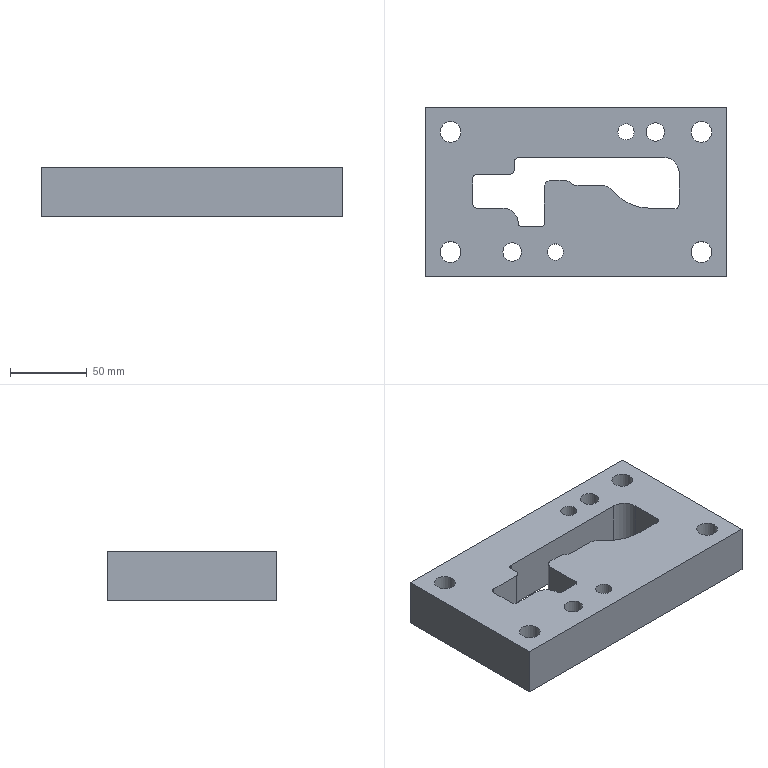Part | STEP file | lll_id226_x_t | 1 solid | 49 faces | box 195 x 110 x 32 mm | volume 531719 mm3 | cylinder 27 | plane 22 | commonest cylinder face diameters 6 x6 13.509 x4 20.008 x4 4 x2 8 x2 10.505 x2
STEP:
#1=CARTESIAN_POINT('',(1138.753,9.,60.5));
#2=VERTEX_POINT('',#1);
#3=CARTESIAN_POINT('',(1133.5,9.,60.5));
#4=DIRECTION('',(0.,0.,1.));
#5=DIRECTION('',(1.,0.,0.));
#6=AXIS2_PLACEMENT_3D('',#3,#4,#5);
#7=CIRCLE('',#6,5.253);
#8=EDGE_CURVE('',#2,#2,#7,.T.);
#9=ORIENTED_EDGE('',*,*,#8,.T.);
#10=EDGE_LOOP('',(#9));
#11=FACE_BOUND('',#10,.T.);
#12=CARTESIAN_POINT('',(1065.5,-69.,60.5));
#13=VERTEX_POINT('',#12);
#14=CARTESIAN_POINT('',(1059.5,-69.,60.5));
#15=DIRECTION('',(0.,0.,-1.));
#16=DIRECTION('',(1.,0.,0.));
#17=AXIS2_PLACEMENT_3D('',#14,#15,#16);
#18=CIRCLE('',#17,6.);
#19=EDGE_CURVE('',#13,#13,#18,.T.);
#20=ORIENTED_EDGE('',*,*,#19,.F.);
#21=EDGE_LOOP('',(#20));
#22=FACE_BOUND('',#21,.T.);
#23=CARTESIAN_POINT('',(1158.5,9.,60.5));
#24=VERTEX_POINT('',#23);
#25=CARTESIAN_POINT('',(1152.5,9.,60.5));
#26=DIRECTION('',(0.,0.,-1.));
#27=DIRECTION('',(1.,0.,0.));
#28=AXIS2_PLACEMENT_3D('',#25,#26,#27);
#29=CIRCLE('',#28,6.);
#30=EDGE_CURVE('',#24,#24,#29,.T.);
#31=ORIENTED_EDGE('',*,*,#30,.F.);
#32=EDGE_LOOP('',(#31));
#33=FACE_BOUND('',#32,.T.);
#34=CARTESIAN_POINT('',(1009.496,9.,60.5));
#35=VERTEX_POINT('',#34);
#36=CARTESIAN_POINT('',(1019.5,9.,60.5));
#37=DIRECTION('',(0.,0.,1.));
#38=DIRECTION('',(-1.,0.,0.));
#39=AXIS2_PLACEMENT_3D('',#36,#37,#38);
#40=CIRCLE('',#39,10.004);
#41=EDGE_CURVE('',#35,#35,#40,.T.);
#42=ORIENTED_EDGE('',*,*,#41,.T.);
#43=EDGE_LOOP('',(#42));
#44=FACE_BOUND('',#43,.T.);
#45=CARTESIAN_POINT('',(1172.496,9.,60.5));
#46=VERTEX_POINT('',#45);
#47=CARTESIAN_POINT('',(1182.5,9.,60.5));
#48=DIRECTION('',(0.,0.,1.));
#49=DIRECTION('',(-1.,0.,0.));
#50=AXIS2_PLACEMENT_3D('',#47,#48,#49);
#51=CIRCLE('',#50,10.004);
#52=EDGE_CURVE('',#46,#46,#51,.T.);
#53=ORIENTED_EDGE('',*,*,#52,.T.);
#54=EDGE_LOOP('',(#53));
#55=FACE_BOUND('',#54,.T.);
#56=CARTESIAN_POINT('',(1003.5,25.,60.5));
#57=VERTEX_POINT('',#56);
#58=CARTESIAN_POINT('',(1003.5,-85.,60.5));
#59=VERTEX_POINT('',#58);
#60=CARTESIAN_POINT('',(1003.5,-30.,60.5));
#61=DIRECTION('',(0.,-1.,0.));
#62=VECTOR('',#61,1.);
#63=LINE('',#60,#62);
#64=EDGE_CURVE('',#57,#59,#63,.T.);
#65=ORIENTED_EDGE('',*,*,#64,.F.);
#66=CARTESIAN_POINT('',(1198.5,25.,60.5));
#67=VERTEX_POINT('',#66);
#68=CARTESIAN_POINT('',(1101.,25.,60.5));
#69=DIRECTION('',(-1.,0.,0.));
#70=VECTOR('',#69,1.);
#71=LINE('',#68,#70);
#72=EDGE_CURVE('',#67,#57,#71,.T.);
#73=ORIENTED_EDGE('',*,*,#72,.F.);
#74=CARTESIAN_POINT('',(1198.5,-85.,60.5));
#75=VERTEX_POINT('',#74);
#76=CARTESIAN_POINT('',(1198.5,-30.,60.5));
#77=DIRECTION('',(0.,1.,0.));
#78=VECTOR('',#77,1.);
#79=LINE('',#76,#78);
#80=EDGE_CURVE('',#75,#67,#79,.T.);
#81=ORIENTED_EDGE('',*,*,#80,.F.);
#82=CARTESIAN_POINT('',(1101.,-85.,60.5));
#83=DIRECTION('',(1.,0.,0.));
#84=VECTOR('',#83,1.);
#85=LINE('',#82,#84);
#86=EDGE_CURVE('',#59,#75,#85,.T.);
#87=ORIENTED_EDGE('',*,*,#86,.F.);
#88=EDGE_LOOP('',(#65,#73,#81,#87));
#89=FACE_BOUND('',#88,.T.);
#90=CARTESIAN_POINT('',(1009.496,-69.,60.5));
#91=VERTEX_POINT('',#90);
#92=CARTESIAN_POINT('',(1019.5,-69.,60.5));
#93=DIRECTION('',(0.,0.,1.));
#94=DIRECTION('',(-1.,0.,0.));
#95=AXIS2_PLACEMENT_3D('',#92,#93,#94);
#96=CIRCLE('',#95,10.004);
#97=EDGE_CURVE('',#91,#91,#96,.T.);
#98=ORIENTED_EDGE('',*,*,#97,.T.);
#99=EDGE_LOOP('',(#98));
#100=FACE_BOUND('',#99,.T.);
#101=CARTESIAN_POINT('',(1172.496,-69.,60.5));
#102=VERTEX_POINT('',#101);
#103=CARTESIAN_POINT('',(1182.5,-69.,60.5));
#104=DIRECTION('',(0.,0.,1.));
#105=DIRECTION('',(-1.,0.,0.));
#106=AXIS2_PLACEMENT_3D('',#103,#104,#105);
#107=CIRCLE('',#106,10.004);
#108=EDGE_CURVE('',#102,#102,#107,.T.);
#109=ORIENTED_EDGE('',*,*,#108,.T.);
#110=EDGE_LOOP('',(#109));
#111=FACE_BOUND('',#110,.T.);
#112=CARTESIAN_POINT('',(1092.753,-69.,60.5));
#113=VERTEX_POINT('',#112);
#114=CARTESIAN_POINT('',(1087.5,-69.,60.5));
#115=DIRECTION('',(0.,0.,1.));
#116=DIRECTION('',(1.,0.,0.));
#117=AXIS2_PLACEMENT_3D('',#114,#115,#116);
#118=CIRCLE('',#117,5.253);
#119=EDGE_CURVE('',#113,#113,#118,.T.);
#120=ORIENTED_EDGE('',*,*,#119,.T.);
#121=EDGE_LOOP('',(#120));
#122=FACE_BOUND('',#121,.T.);
#123=CARTESIAN_POINT('',(1158.,-7.5,60.5));
#124=VERTEX_POINT('',#123);
#125=CARTESIAN_POINT('',(1168.,-17.5,60.5));
#126=VERTEX_POINT('',#125);
#127=CARTESIAN_POINT('',(1158.,-17.5,60.5));
#128=DIRECTION('',(0.,0.,-1.));
#129=DIRECTION('',(-1.,0.,0.));
#130=AXIS2_PLACEMENT_3D('',#127,#128,#129);
#131=CIRCLE('',#130,10.);
#132=EDGE_CURVE('',#124,#126,#131,.T.);
#133=ORIENTED_EDGE('',*,*,#132,.F.);
#134=CARTESIAN_POINT('',(1064.,-7.5,60.5));
#135=VERTEX_POINT('',#134);
#136=CARTESIAN_POINT('',(1101.,-7.5,60.5));
#137=DIRECTION('',(1.,0.,0.));
#138=VECTOR('',#137,1.);
#139=LINE('',#136,#138);
#140=EDGE_CURVE('',#135,#124,#139,.T.);
#141=ORIENTED_EDGE('',*,*,#140,.F.);
#142=CARTESIAN_POINT('',(1061.,-10.5,60.5));
#143=VERTEX_POINT('',#142);
#144=CARTESIAN_POINT('',(1064.,-10.5,60.5));
#145=DIRECTION('',(0.,0.,-1.));
#146=DIRECTION('',(-1.,0.,0.));
#147=AXIS2_PLACEMENT_3D('',#144,#145,#146);
#148=CIRCLE('',#147,3.);
#149=EDGE_CURVE('',#143,#135,#148,.T.);
#150=ORIENTED_EDGE('',*,*,#149,.F.);
#151=CARTESIAN_POINT('',(1061.,-15.5,60.5));
#152=VERTEX_POINT('',#151);
#153=CARTESIAN_POINT('',(1061.,-30.,60.5));
#154=DIRECTION('',(0.,1.,0.));
#155=VECTOR('',#154,1.);
#156=LINE('',#153,#155);
#157=EDGE_CURVE('',#152,#143,#156,.T.);
#158=ORIENTED_EDGE('',*,*,#157,.F.);
#159=CARTESIAN_POINT('',(1058.,-18.5,60.5));
#160=VERTEX_POINT('',#159);
#161=CARTESIAN_POINT('',(1058.,-15.5,60.5));
#162=DIRECTION('',(0.,0.,1.));
#163=DIRECTION('',(-1.,0.,0.));
#164=AXIS2_PLACEMENT_3D('',#161,#162,#163);
#165=CIRCLE('',#164,3.);
#166=EDGE_CURVE('',#160,#152,#165,.T.);
#167=ORIENTED_EDGE('',*,*,#166,.F.);
#168=CARTESIAN_POINT('',(1037.,-18.5,60.5));
#169=VERTEX_POINT('',#168);
#170=CARTESIAN_POINT('',(1101.,-18.5,60.5));
#171=DIRECTION('',(1.,0.,0.));
#172=VECTOR('',#171,1.);
#173=LINE('',#170,#172);
#174=EDGE_CURVE('',#169,#160,#173,.T.);
#175=ORIENTED_EDGE('',*,*,#174,.F.);
#176=CARTESIAN_POINT('',(1034.,-21.5,60.5));
#177=VERTEX_POINT('',#176);
#178=CARTESIAN_POINT('',(1037.,-21.5,60.5));
#179=DIRECTION('',(0.,0.,-1.));
#180=DIRECTION('',(-1.,0.,0.));
#181=AXIS2_PLACEMENT_3D('',#178,#179,#180);
#182=CIRCLE('',#181,3.);
#183=EDGE_CURVE('',#177,#169,#182,.T.);
#184=ORIENTED_EDGE('',*,*,#183,.F.);
#185=CARTESIAN_POINT('',(1034.,-37.5,60.5));
#186=VERTEX_POINT('',#185);
#187=CARTESIAN_POINT('',(1034.,-30.,60.5));
#188=DIRECTION('',(0.,-1.,0.));
#189=VECTOR('',#188,1.);
#190=LINE('',#187,#189);
#191=EDGE_CURVE('',#177,#186,#190,.T.);
#192=ORIENTED_EDGE('',*,*,#191,.T.);
#193=CARTESIAN_POINT('',(1037.,-40.5,60.5));
#194=VERTEX_POINT('',#193);
#195=CARTESIAN_POINT('',(1037.,-37.5,60.5));
#196=DIRECTION('',(0.,0.,1.));
#197=DIRECTION('',(-1.,0.,0.));
#198=AXIS2_PLACEMENT_3D('',#195,#196,#197);
#199=CIRCLE('',#198,3.);
#200=EDGE_CURVE('',#186,#194,#199,.T.);
#201=ORIENTED_EDGE('',*,*,#200,.T.);
#202=CARTESIAN_POINT('',(1053.5,-40.5,60.5));
#203=VERTEX_POINT('',#202);
#204=CARTESIAN_POINT('',(1101.,-40.5,60.5));
#205=DIRECTION('',(1.,0.,0.));
#206=VECTOR('',#205,1.);
#207=LINE('',#204,#206);
#208=EDGE_CURVE('',#194,#203,#207,.T.);
#209=ORIENTED_EDGE('',*,*,#208,.T.);
#210=CARTESIAN_POINT('',(1063.5,-50.5,60.5));
#211=VERTEX_POINT('',#210);
#212=CARTESIAN_POINT('',(1053.499,-50.501,60.5));
#213=DIRECTION('',(0.,0.,1.));
#214=DIRECTION('',(-1.,0.,0.));
#215=AXIS2_PLACEMENT_3D('',#212,#213,#214);
#216=CIRCLE('',#215,10.001);
#217=EDGE_CURVE('',#211,#203,#216,.T.);
#218=ORIENTED_EDGE('',*,*,#217,.F.);
#219=CARTESIAN_POINT('',(1065.5,-52.5,60.5));
#220=VERTEX_POINT('',#219);
#221=CARTESIAN_POINT('',(1065.5,-50.5,60.5));
#222=DIRECTION('',(0.,0.,-1.));
#223=DIRECTION('',(-1.,0.,0.));
#224=AXIS2_PLACEMENT_3D('',#221,#222,#223);
#225=CIRCLE('',#224,2.);
#226=EDGE_CURVE('',#220,#211,#225,.T.);
#227=ORIENTED_EDGE('',*,*,#226,.F.);
#228=CARTESIAN_POINT('',(1078.51,-52.5,60.5));
#229=VERTEX_POINT('',#228);
#230=CARTESIAN_POINT('',(1101.,-52.5,60.5));
#231=DIRECTION('',(-1.,0.,0.));
#232=VECTOR('',#231,1.);
#233=LINE('',#230,#232);
#234=EDGE_CURVE('',#229,#220,#233,.T.);
#235=ORIENTED_EDGE('',*,*,#234,.F.);
#236=CARTESIAN_POINT('',(1080.51,-50.5,60.5));
#237=VERTEX_POINT('',#236);
#238=CARTESIAN_POINT('',(1078.51,-50.5,60.5));
#239=DIRECTION('',(0.,0.,-1.));
#240=DIRECTION('',(-1.,0.,0.));
#241=AXIS2_PLACEMENT_3D('',#238,#239,#240);
#242=CIRCLE('',#241,2.);
#243=EDGE_CURVE('',#237,#229,#242,.T.);
#244=ORIENTED_EDGE('',*,*,#243,.F.);
#245=CARTESIAN_POINT('',(1080.512,-26.495,60.5));
#246=VERTEX_POINT('',#245);
#247=CARTESIAN_POINT('',(1080.512,-29.999,60.5));
#248=DIRECTION('',(0.00006142,1.,0.));
#249=VECTOR('',#248,1.);
#250=LINE('',#247,#249);
#251=EDGE_CURVE('',#237,#246,#250,.T.);
#252=ORIENTED_EDGE('',*,*,#251,.T.);
#253=CARTESIAN_POINT('',(1084.513,-22.495,60.5));
#254=VERTEX_POINT('',#253);
#255=CARTESIAN_POINT('',(1084.512,-26.495,60.5));
#256=DIRECTION('',(0.,0.,-1.));
#257=DIRECTION('',(-1.,0.,0.));
#258=AXIS2_PLACEMENT_3D('',#255,#256,#257);
#259=CIRCLE('',#258,4.);
#260=EDGE_CURVE('',#246,#254,#259,.T.);
#261=ORIENTED_EDGE('',*,*,#260,.T.);
#262=CARTESIAN_POINT('',(1094.017,-22.497,60.5));
#263=VERTEX_POINT('',#262);
#264=CARTESIAN_POINT('',(1101.001,-22.498,60.5));
#265=DIRECTION('',(1.,-0.0001728,0.));
#266=VECTOR('',#265,1.);
#267=LINE('',#264,#266);
#268=EDGE_CURVE('',#254,#263,#267,.T.);
#269=ORIENTED_EDGE('',*,*,#268,.T.);
#270=CARTESIAN_POINT('',(1097.128,-23.983,60.5));
#271=VERTEX_POINT('',#270);
#272=CARTESIAN_POINT('',(1094.016,-26.497,60.5));
#273=DIRECTION('',(0.,0.,1.));
#274=DIRECTION('',(-1.,0.,0.));
#275=AXIS2_PLACEMENT_3D('',#272,#273,#274);
#276=CIRCLE('',#275,4.);
#277=EDGE_CURVE('',#271,#263,#276,.T.);
#278=ORIENTED_EDGE('',*,*,#277,.F.);
#279=CARTESIAN_POINT('',(1100.313,-25.498,60.5));
#280=VERTEX_POINT('',#279);
#281=CARTESIAN_POINT('',(1100.299,-21.422,60.5));
#282=DIRECTION('',(0.,0.,-1.));
#283=DIRECTION('',(-1.,0.,0.));
#284=AXIS2_PLACEMENT_3D('',#281,#282,#283);
#285=CIRCLE('',#284,4.076);
#286=EDGE_CURVE('',#280,#271,#285,.T.);
#287=ORIENTED_EDGE('',*,*,#286,.F.);
#288=CARTESIAN_POINT('',(1116.863,-25.503,60.5));
#289=VERTEX_POINT('',#288);
#290=CARTESIAN_POINT('',(1101.001,-25.498,60.5));
#291=DIRECTION('',(1.,-0.0002888,0.));
#292=VECTOR('',#291,1.);
#293=LINE('',#290,#292);
#294=EDGE_CURVE('',#280,#289,#293,.T.);
#295=ORIENTED_EDGE('',*,*,#294,.T.);
#296=CARTESIAN_POINT('',(1123.932,-28.432,60.5));
#297=VERTEX_POINT('',#296);
#298=CARTESIAN_POINT('',(1116.86,-35.503,60.5));
#299=DIRECTION('',(0.,0.,1.));
#300=DIRECTION('',(-1.,0.,0.));
#301=AXIS2_PLACEMENT_3D('',#298,#299,#300);
#302=CIRCLE('',#301,10.);
#303=EDGE_CURVE('',#297,#289,#302,.T.);
#304=ORIENTED_EDGE('',*,*,#303,.F.);
#305=CARTESIAN_POINT('',(1127.213,-31.713,60.5));
#306=VERTEX_POINT('',#305);
#307=CARTESIAN_POINT('',(1113.25,-17.75,60.5));
#308=DIRECTION('',(0.7071,-0.7071,0.));
#309=VECTOR('',#308,1.);
#310=LINE('',#307,#309);
#311=EDGE_CURVE('',#297,#306,#310,.T.);
#312=ORIENTED_EDGE('',*,*,#311,.T.);
#313=CARTESIAN_POINT('',(1148.426,-40.5,60.5));
#314=VERTEX_POINT('',#313);
#315=CARTESIAN_POINT('',(1148.426,-10.502,60.5));
#316=DIRECTION('',(0.,0.,1.));
#317=DIRECTION('',(-1.,0.,0.));
#318=AXIS2_PLACEMENT_3D('',#315,#316,#317);
#319=CIRCLE('',#318,29.998);
#320=EDGE_CURVE('',#306,#314,#319,.T.);
#321=ORIENTED_EDGE('',*,*,#320,.T.);
#322=CARTESIAN_POINT('',(1162.602,-40.5,60.5));
#323=VERTEX_POINT('',#322);
#324=CARTESIAN_POINT('',(1101.,-40.5,60.5));
#325=DIRECTION('',(-1.,0.,0.));
#326=VECTOR('',#325,1.);
#327=LINE('',#324,#326);
#328=EDGE_CURVE('',#323,#314,#327,.T.);
#329=ORIENTED_EDGE('',*,*,#328,.F.);
#330=CARTESIAN_POINT('',(1163.801,-40.75,60.5));
#331=VERTEX_POINT('',#330);
#332=CARTESIAN_POINT('',(1162.602,-43.5,60.5));
#333=DIRECTION('',(0.,0.,-1.));
#334=DIRECTION('',(-1.,0.,0.));
#335=AXIS2_PLACEMENT_3D('',#332,#333,#334);
#336=CIRCLE('',#335,3.);
#337=EDGE_CURVE('',#323,#331,#336,.T.);
#338=ORIENTED_EDGE('',*,*,#337,.T.);
#339=CARTESIAN_POINT('',(1168.,-38.,60.5));
#340=VERTEX_POINT('',#339);
#341=CARTESIAN_POINT('',(1165.,-38.,60.5));
#342=DIRECTION('',(0.,0.,1.));
#343=DIRECTION('',(-1.,0.,0.));
#344=AXIS2_PLACEMENT_3D('',#341,#342,#343);
#345=CIRCLE('',#344,3.);
#346=EDGE_CURVE('',#331,#340,#345,.T.);
#347=ORIENTED_EDGE('',*,*,#346,.T.);
#348=CARTESIAN_POINT('',(1168.,-30.,60.5));
#349=DIRECTION('',(0.,-1.,0.));
#350=VECTOR('',#349,1.);
#351=LINE('',#348,#350);
#352=EDGE_CURVE('',#126,#340,#351,.T.);
#353=ORIENTED_EDGE('',*,*,#352,.F.);
#354=EDGE_LOOP('',(#133,#141,#150,#158,#167,#175,#184,#192,#201,#209,#218,#227,#235,#244,#252,#261,#269,#278,#287,#295,#304,#312,#321,#329,#338,#347,#353));
#355=FACE_BOUND('',#354,.T.);
#356=CARTESIAN_POINT('',(1101.,-30.,60.5));
#357=DIRECTION('',(0.,0.,-1.));
#358=DIRECTION('',(1.,0.,0.));
#359=AXIS2_PLACEMENT_3D('',#356,#357,#358);
#360=PLANE('',#359);
#361=ADVANCED_FACE('',(#11,#22,#33,#44,#55,#89,#100,#111,#122,#355),#360,.T.);
#362=CARTESIAN_POINT('',(1003.5,25.,92.5));
#363=VERTEX_POINT('',#362);
#364=CARTESIAN_POINT('',(1198.5,25.,92.5));
#365=VERTEX_POINT('',#364);
#366=CARTESIAN_POINT('',(1101.,25.,92.5));
#367=DIRECTION('',(1.,0.,0.));
#368=VECTOR('',#367,1.);
#369=LINE('',#366,#368);
#370=EDGE_CURVE('',#363,#365,#369,.T.);
#371=ORIENTED_EDGE('',*,*,#370,.F.);
#372=CARTESIAN_POINT('',(1003.5,-85.,92.5));
#373=VERTEX_POINT('',#372);
#374=CARTESIAN_POINT('',(1003.5,-30.,92.5));
#375=DIRECTION('',(0.,1.,0.));
#376=VECTOR('',#375,1.);
#377=LINE('',#374,#376);
#378=EDGE_CURVE('',#373,#363,#377,.T.);
#379=ORIENTED_EDGE('',*,*,#378,.F.);
#380=CARTESIAN_POINT('',(1198.5,-85.,92.5));
#381=VERTEX_POINT('',#380);
#382=CARTESIAN_POINT('',(1101.,-85.,92.5));
#383=DIRECTION('',(-1.,0.,0.));
#384=VECTOR('',#383,1.);
#385=LINE('',#382,#384);
#386=EDGE_CURVE('',#381,#373,#385,.T.);
#387=ORIENTED_EDGE('',*,*,#386,.F.);
#388=CARTESIAN_POINT('',(1198.5,-30.,92.5));
#389=DIRECTION('',(0.,-1.,0.));
#390=VECTOR('',#389,1.);
#391=LINE('',#388,#390);
#392=EDGE_CURVE('',#365,#381,#391,.T.);
#393=ORIENTED_EDGE('',*,*,#392,.F.);
#394=EDGE_LOOP('',(#371,#379,#387,#393));
#395=FACE_BOUND('',#394,.T.);
#396=CARTESIAN_POINT('',(1175.745,9.,92.5));
#397=VERTEX_POINT('',#396);
#398=CARTESIAN_POINT('',(1182.5,9.,92.5));
#399=DIRECTION('',(0.,0.,1.));
#400=DIRECTION('',(-1.,0.,0.));
#401=AXIS2_PLACEMENT_3D('',#398,#399,#400);
#402=CIRCLE('',#401,6.755);
#403=EDGE_CURVE('',#397,#397,#402,.T.);
#404=ORIENTED_EDGE('',*,*,#403,.F.);
#405=EDGE_LOOP('',(#404));
#406=FACE_BOUND('',#405,.T.);
#407=CARTESIAN_POINT('',(1012.745,-69.,92.5));
#408=VERTEX_POINT('',#407);
#409=CARTESIAN_POINT('',(1019.5,-69.,92.5));
#410=DIRECTION('',(0.,0.,1.));
#411=DIRECTION('',(-1.,0.,0.));
#412=AXIS2_PLACEMENT_3D('',#409,#410,#411);
#413=CIRCLE('',#412,6.755);
#414=EDGE_CURVE('',#408,#408,#413,.T.);
#415=ORIENTED_EDGE('',*,*,#414,.F.);
#416=EDGE_LOOP('',(#415));
#417=FACE_BOUND('',#416,.T.);
#418=CARTESIAN_POINT('',(1012.745,9.,92.5));
#419=VERTEX_POINT('',#418);
#420=CARTESIAN_POINT('',(1019.5,9.,92.5));
#421=DIRECTION('',(0.,0.,1.));
#422=DIRECTION('',(-1.,0.,0.));
#423=AXIS2_PLACEMENT_3D('',#420,#421,#422);
#424=CIRCLE('',#423,6.755);
#425=EDGE_CURVE('',#419,#419,#424,.T.);
#426=ORIENTED_EDGE('',*,*,#425,.F.);
#427=EDGE_LOOP('',(#426));
#428=FACE_BOUND('',#427,.T.);
#429=CARTESIAN_POINT('',(1175.745,-69.,92.5));
#430=VERTEX_POINT('',#429);
#431=CARTESIAN_POINT('',(1182.5,-69.,92.5));
#432=DIRECTION('',(0.,0.,1.));
#433=DIRECTION('',(-1.,0.,0.));
#434=AXIS2_PLACEMENT_3D('',#431,#432,#433);
#435=CIRCLE('',#434,6.755);
#436=EDGE_CURVE('',#430,#430,#435,.T.);
#437=ORIENTED_EDGE('',*,*,#436,.F.);
#438=EDGE_LOOP('',(#437));
#439=FACE_BOUND('',#438,.T.);
#440=CARTESIAN_POINT('',(1146.5,9.,92.5));
#441=VERTEX_POINT('',#440);
#442=CARTESIAN_POINT('',(1152.5,9.,92.5));
#443=DIRECTION('',(0.,0.,1.));
#444=DIRECTION('',(-1.,0.,0.));
#445=AXIS2_PLACEMENT_3D('',#442,#443,#444);
#446=CIRCLE('',#445,6.);
#447=EDGE_CURVE('',#441,#441,#446,.T.);
#448=ORIENTED_EDGE('',*,*,#447,.F.);
#449=EDGE_LOOP('',(#448));
#450=FACE_BOUND('',#449,.T.);
#451=CARTESIAN_POINT('',(1053.5,-69.,92.5));
#452=VERTEX_POINT('',#451);
#453=CARTESIAN_POINT('',(1059.5,-69.,92.5));
#454=DIRECTION('',(0.,0.,1.));
#455=DIRECTION('',(-1.,0.,0.));
#456=AXIS2_PLACEMENT_3D('',#453,#454,#455);
#457=CIRCLE('',#456,6.);
#458=EDGE_CURVE('',#452,#452,#457,.T.);
#459=ORIENTED_EDGE('',*,*,#458,.F.);
#460=EDGE_LOOP('',(#459));
#461=FACE_BOUND('',#460,.T.);
#462=CARTESIAN_POINT('',(1138.753,9.,92.5));
#463=VERTEX_POINT('',#462);
#464=CARTESIAN_POINT('',(1133.5,9.,92.5));
#465=DIRECTION('',(0.,0.,1.));
#466=DIRECTION('',(1.,0.,0.));
#467=AXIS2_PLACEMENT_3D('',#464,#465,#466);
#468=CIRCLE('',#467,5.253);
#469=EDGE_CURVE('',#463,#463,#468,.T.);
#470=ORIENTED_EDGE('',*,*,#469,.F.);
#471=EDGE_LOOP('',(#470));
#472=FACE_BOUND('',#471,.T.);
#473=CARTESIAN_POINT('',(1092.753,-69.,92.5));
#474=VERTEX_POINT('',#473);
#475=CARTESIAN_POINT('',(1087.5,-69.,92.5));
#476=DIRECTION('',(0.,0.,1.));
#477=DIRECTION('',(1.,0.,0.));
#478=AXIS2_PLACEMENT_3D('',#475,#476,#477);
#479=CIRCLE('',#478,5.253);
#480=EDGE_CURVE('',#474,#474,#479,.T.);
#481=ORIENTED_EDGE('',*,*,#480,.F.);
#482=EDGE_LOOP('',(#481));
#483=FACE_BOUND('',#482,.T.);
#484=CARTESIAN_POINT('',(1061.,-10.5,92.5));
#485=VERTEX_POINT('',#484);
#486=CARTESIAN_POINT('',(1064.,-7.5,92.5));
#487=VERTEX_POINT('',#486);
#488=CARTESIAN_POINT('',(1064.,-10.5,92.5));
#489=DIRECTION('',(0.,0.,-1.));
#490=DIRECTION('',(1.,0.,0.));
#491=AXIS2_PLACEMENT_3D('',#488,#489,#490);
#492=CIRCLE('',#491,3.);
#493=EDGE_CURVE('',#485,#487,#492,.T.);
#494=ORIENTED_EDGE('',*,*,#493,.T.);
#495=CARTESIAN_POINT('',(1158.,-7.5,92.5));
#496=VERTEX_POINT('',#495);
#497=CARTESIAN_POINT('',(1101.,-7.5,92.5));
#498=DIRECTION('',(1.,0.,0.));
#499=VECTOR('',#498,1.);
#500=LINE('',#497,#499);
#501=EDGE_CURVE('',#487,#496,#500,.T.);
#502=ORIENTED_EDGE('',*,*,#501,.T.);
#503=CARTESIAN_POINT('',(1168.,-17.5,92.5));
#504=VERTEX_POINT('',#503);
#505=CARTESIAN_POINT('',(1158.,-17.5,92.5));
#506=DIRECTION('',(0.,0.,1.));
#507=DIRECTION('',(1.,0.,0.));
#508=AXIS2_PLACEMENT_3D('',#505,#506,#507);
#509=CIRCLE('',#508,10.);
#510=EDGE_CURVE('',#504,#496,#509,.T.);
#511=ORIENTED_EDGE('',*,*,#510,.F.);
#512=CARTESIAN_POINT('',(1168.,-38.,92.5));
#513=VERTEX_POINT('',#512);
#514=CARTESIAN_POINT('',(1168.,-30.,92.5));
#515=DIRECTION('',(0.,-1.,0.));
#516=VECTOR('',#515,1.);
#517=LINE('',#514,#516);
#518=EDGE_CURVE('',#504,#513,#517,.T.);
#519=ORIENTED_EDGE('',*,*,#518,.T.);
#520=CARTESIAN_POINT('',(1163.801,-40.75,92.5));
#521=VERTEX_POINT('',#520);
#522=CARTESIAN_POINT('',(1165.,-38.,92.5));
#523=DIRECTION('',(0.,0.,1.));
#524=DIRECTION('',(1.,0.,0.));
#525=AXIS2_PLACEMENT_3D('',#522,#523,#524);
#526=CIRCLE('',#525,3.);
#527=EDGE_CURVE('',#521,#513,#526,.T.);
#528=ORIENTED_EDGE('',*,*,#527,.F.);
#529=CARTESIAN_POINT('',(1162.602,-40.5,92.5));
#530=VERTEX_POINT('',#529);
#531=CARTESIAN_POINT('',(1162.602,-43.5,92.5));
#532=DIRECTION('',(0.,0.,1.));
#533=DIRECTION('',(1.,0.,0.));
#534=AXIS2_PLACEMENT_3D('',#531,#532,#533);
#535=CIRCLE('',#534,3.);
#536=EDGE_CURVE('',#521,#530,#535,.T.);
#537=ORIENTED_EDGE('',*,*,#536,.T.);
#538=CARTESIAN_POINT('',(1148.426,-40.5,92.5));
#539=VERTEX_POINT('',#538);
#540=CARTESIAN_POINT('',(1101.,-40.5,92.5));
#541=DIRECTION('',(-1.,0.,0.));
#542=VECTOR('',#541,1.);
#543=LINE('',#540,#542);
#544=EDGE_CURVE('',#530,#539,#543,.T.);
#545=ORIENTED_EDGE('',*,*,#544,.T.);
#546=CARTESIAN_POINT('',(1127.213,-31.713,92.5));
#547=VERTEX_POINT('',#546);
#548=CARTESIAN_POINT('',(1148.426,-10.502,92.5));
#549=DIRECTION('',(0.,0.,1.));
#550=DIRECTION('',(1.,0.,0.));
#551=AXIS2_PLACEMENT_3D('',#548,#549,#550);
#552=CIRCLE('',#551,29.998);
#553=EDGE_CURVE('',#547,#539,#552,.T.);
#554=ORIENTED_EDGE('',*,*,#553,.F.);
#555=CARTESIAN_POINT('',(1123.932,-28.432,92.5));
#556=VERTEX_POINT('',#555);
#557=CARTESIAN_POINT('',(1113.25,-17.75,92.5));
#558=DIRECTION('',(-0.7071,0.7071,0.));
#559=VECTOR('',#558,1.);
#560=LINE('',#557,#559);
#561=EDGE_CURVE('',#547,#556,#560,.T.);
#562=ORIENTED_EDGE('',*,*,#561,.T.);
#563=CARTESIAN_POINT('',(1116.863,-25.503,92.5));
#564=VERTEX_POINT('',#563);
#565=CARTESIAN_POINT('',(1116.86,-35.503,92.5));
#566=DIRECTION('',(0.,0.,-1.));
#567=DIRECTION('',(1.,0.,0.));
#568=AXIS2_PLACEMENT_3D('',#565,#566,#567);
#569=CIRCLE('',#568,10.);
#570=EDGE_CURVE('',#564,#556,#569,.T.);
#571=ORIENTED_EDGE('',*,*,#570,.F.);
#572=CARTESIAN_POINT('',(1100.313,-25.498,92.5));
#573=VERTEX_POINT('',#572);
#574=CARTESIAN_POINT('',(1101.001,-25.498,92.5));
#575=DIRECTION('',(-1.,0.0002888,0.));
#576=VECTOR('',#575,1.);
#577=LINE('',#574,#576);
#578=EDGE_CURVE('',#564,#573,#577,.T.);
#579=ORIENTED_EDGE('',*,*,#578,.T.);
#580=CARTESIAN_POINT('',(1097.128,-23.983,92.5));
#581=VERTEX_POINT('',#580);
#582=CARTESIAN_POINT('',(1100.299,-21.422,92.5));
#583=DIRECTION('',(0.,0.,1.));
#584=DIRECTION('',(1.,0.,0.));
#585=AXIS2_PLACEMENT_3D('',#582,#583,#584);
#586=CIRCLE('',#585,4.076);
#587=EDGE_CURVE('',#581,#573,#586,.T.);
#588=ORIENTED_EDGE('',*,*,#587,.F.);
#589=CARTESIAN_POINT('',(1094.017,-22.497,92.5));
#590=VERTEX_POINT('',#589);
#591=CARTESIAN_POINT('',(1094.016,-26.497,92.5));
#592=DIRECTION('',(0.,0.,-1.));
#593=DIRECTION('',(1.,0.,0.));
#594=AXIS2_PLACEMENT_3D('',#591,#592,#593);
#595=CIRCLE('',#594,4.);
#596=EDGE_CURVE('',#590,#581,#595,.T.);
#597=ORIENTED_EDGE('',*,*,#596,.F.);
#598=CARTESIAN_POINT('',(1084.513,-22.495,92.5));
#599=VERTEX_POINT('',#598);
#600=CARTESIAN_POINT('',(1101.001,-22.498,92.5));
#601=DIRECTION('',(-1.,0.0001728,0.));
#602=VECTOR('',#601,1.);
#603=LINE('',#600,#602);
#604=EDGE_CURVE('',#590,#599,#603,.T.);
#605=ORIENTED_EDGE('',*,*,#604,.T.);
#606=CARTESIAN_POINT('',(1080.512,-26.495,92.5));
#607=VERTEX_POINT('',#606);
#608=CARTESIAN_POINT('',(1084.512,-26.495,92.5));
#609=DIRECTION('',(0.,0.,-1.));
#610=DIRECTION('',(1.,0.,0.));
#611=AXIS2_PLACEMENT_3D('',#608,#609,#610);
#612=CIRCLE('',#611,4.);
#613=EDGE_CURVE('',#607,#599,#612,.T.);
#614=ORIENTED_EDGE('',*,*,#613,.F.);
#615=CARTESIAN_POINT('',(1080.51,-50.5,92.5));
#616=VERTEX_POINT('',#615);
#617=CARTESIAN_POINT('',(1080.512,-29.999,92.5));
#618=DIRECTION('',(-0.00006142,-1.,0.));
#619=VECTOR('',#618,1.);
#620=LINE('',#617,#619);
#621=EDGE_CURVE('',#607,#616,#620,.T.);
#622=ORIENTED_EDGE('',*,*,#621,.T.);
#623=CARTESIAN_POINT('',(1078.51,-52.5,92.5));
#624=VERTEX_POINT('',#623);
#625=CARTESIAN_POINT('',(1078.51,-50.5,92.5));
#626=DIRECTION('',(0.,0.,1.));
#627=DIRECTION('',(1.,0.,0.));
#628=AXIS2_PLACEMENT_3D('',#625,#626,#627);
#629=CIRCLE('',#628,2.);
#630=EDGE_CURVE('',#624,#616,#629,.T.);
#631=ORIENTED_EDGE('',*,*,#630,.F.);
#632=CARTESIAN_POINT('',(1065.5,-52.5,92.5));
#633=VERTEX_POINT('',#632);
#634=CARTESIAN_POINT('',(1101.,-52.5,92.5));
#635=DIRECTION('',(-1.,0.,0.));
#636=VECTOR('',#635,1.);
#637=LINE('',#634,#636);
#638=EDGE_CURVE('',#624,#633,#637,.T.);
#639=ORIENTED_EDGE('',*,*,#638,.T.);
#640=CARTESIAN_POINT('',(1063.5,-50.5,92.5));
#641=VERTEX_POINT('',#640);
#642=CARTESIAN_POINT('',(1065.5,-50.5,92.5));
#643=DIRECTION('',(0.,0.,1.));
#644=DIRECTION('',(1.,0.,0.));
#645=AXIS2_PLACEMENT_3D('',#642,#643,#644);
#646=CIRCLE('',#645,2.);
#647=EDGE_CURVE('',#641,#633,#646,.T.);
#648=ORIENTED_EDGE('',*,*,#647,.F.);
#649=CARTESIAN_POINT('',(1053.5,-40.5,92.5));
#650=VERTEX_POINT('',#649);
#651=CARTESIAN_POINT('',(1053.499,-50.501,92.5));
#652=DIRECTION('',(0.,0.,-1.));
#653=DIRECTION('',(1.,0.,0.));
#654=AXIS2_PLACEMENT_3D('',#651,#652,#653);
#655=CIRCLE('',#654,10.001);
#656=EDGE_CURVE('',#650,#641,#655,.T.);
#657=ORIENTED_EDGE('',*,*,#656,.F.);
#658=CARTESIAN_POINT('',(1037.,-40.5,92.5));
#659=VERTEX_POINT('',#658);
#660=CARTESIAN_POINT('',(1101.,-40.5,92.5));
#661=DIRECTION('',(-1.,0.,0.));
#662=VECTOR('',#661,1.);
#663=LINE('',#660,#662);
#664=EDGE_CURVE('',#650,#659,#663,.T.);
#665=ORIENTED_EDGE('',*,*,#664,.T.);
#666=CARTESIAN_POINT('',(1034.,-37.5,92.5));
#667=VERTEX_POINT('',#666);
#668=CARTESIAN_POINT('',(1037.,-37.5,92.5));
#669=DIRECTION('',(0.,0.,1.));
#670=DIRECTION('',(1.,0.,0.));
#671=AXIS2_PLACEMENT_3D('',#668,#669,#670);
#672=CIRCLE('',#671,3.);
#673=EDGE_CURVE('',#667,#659,#672,.T.);
#674=ORIENTED_EDGE('',*,*,#673,.F.);
#675=CARTESIAN_POINT('',(1034.,-21.5,92.5));
#676=VERTEX_POINT('',#675);
#677=CARTESIAN_POINT('',(1034.,-30.,92.5));
#678=DIRECTION('',(0.,1.,0.));
#679=VECTOR('',#678,1.);
#680=LINE('',#677,#679);
#681=EDGE_CURVE('',#667,#676,#680,.T.);
#682=ORIENTED_EDGE('',*,*,#681,.T.);
#683=CARTESIAN_POINT('',(1037.,-18.5,92.5));
#684=VERTEX_POINT('',#683);
#685=CARTESIAN_POINT('',(1037.,-21.5,92.5));
#686=DIRECTION('',(0.,0.,1.));
#687=DIRECTION('',(1.,0.,0.));
#688=AXIS2_PLACEMENT_3D('',#685,#686,#687);
#689=CIRCLE('',#688,3.);
#690=EDGE_CURVE('',#684,#676,#689,.T.);
#691=ORIENTED_EDGE('',*,*,#690,.F.);
#692=CARTESIAN_POINT('',(1058.,-18.5,92.5));
#693=VERTEX_POINT('',#692);
#694=CARTESIAN_POINT('',(1101.,-18.5,92.5));
#695=DIRECTION('',(1.,0.,0.));
#696=VECTOR('',#695,1.);
#697=LINE('',#694,#696);
#698=EDGE_CURVE('',#684,#693,#697,.T.);
#699=ORIENTED_EDGE('',*,*,#698,.T.);
#700=CARTESIAN_POINT('',(1061.,-15.5,92.5));
#701=VERTEX_POINT('',#700);
#702=CARTESIAN_POINT('',(1058.,-15.5,92.5));
#703=DIRECTION('',(0.,0.,-1.));
#704=DIRECTION('',(1.,0.,0.));
#705=AXIS2_PLACEMENT_3D('',#702,#703,#704);
#706=CIRCLE('',#705,3.);
#707=EDGE_CURVE('',#701,#693,#706,.T.);
#708=ORIENTED_EDGE('',*,*,#707,.F.);
#709=CARTESIAN_POINT('',(1061.,-30.,92.5));
#710=DIRECTION('',(0.,1.,0.));
#711=VECTOR('',#710,1.);
#712=LINE('',#709,#711);
#713=EDGE_CURVE('',#701,#485,#712,.T.);
#714=ORIENTED_EDGE('',*,*,#713,.T.);
#715=EDGE_LOOP('',(#494,#502,#511,#519,#528,#537,#545,#554,#562,#571,#579,#588,#597,#605,#614,#622,#631,#639,#648,#657,#665,#674,#682,#691,#699,#708,#714));
#716=FACE_BOUND('',#715,.T.);
#717=CARTESIAN_POINT('',(1101.,-30.,92.5));
#718=DIRECTION('',(0.,0.,1.));
#719=DIRECTION('',(-1.,0.,0.));
#720=AXIS2_PLACEMENT_3D('',#717,#718,#719);
#721=PLANE('',#720);
#722=ADVANCED_FACE('',(#395,#406,#417,#428,#439,#450,#461,#472,#483,#716),#721,.T.);
#723=CARTESIAN_POINT('',(1003.5,25.,60.5));
#724=DIRECTION('',(0.,0.,1.));
#725=VECTOR('',#724,1.);
#726=LINE('',#723,#725);
#727=EDGE_CURVE('',#57,#363,#726,.T.);
#728=ORIENTED_EDGE('',*,*,#727,.T.);
#729=ORIENTED_EDGE('',*,*,#370,.T.);
#730=CARTESIAN_POINT('',(1198.5,25.,60.5));
#731=DIRECTION('',(0.,0.,1.));
#732=VECTOR('',#731,1.);
#733=LINE('',#730,#732);
#734=EDGE_CURVE('',#67,#365,#733,.T.);
#735=ORIENTED_EDGE('',*,*,#734,.F.);
#736=ORIENTED_EDGE('',*,*,#72,.T.);
#737=EDGE_LOOP('',(#728,#729,#735,#736));
#738=FACE_OUTER_BOUND('',#737,.T.);
#739=CARTESIAN_POINT('',(1101.,25.,60.5));
#740=DIRECTION('',(0.,1.,0.));
#741=DIRECTION('',(0.,0.,-1.));
#742=AXIS2_PLACEMENT_3D('',#739,#740,#741);
#743=PLANE('',#742);
#744=ADVANCED_FACE('',(#738),#743,.T.);
#745=ORIENTED_EDGE('',*,*,#734,.T.);
#746=ORIENTED_EDGE('',*,*,#392,.T.);
#747=CARTESIAN_POINT('',(1198.5,-85.,60.5));
#748=DIRECTION('',(0.,0.,1.));
#749=VECTOR('',#748,1.);
#750=LINE('',#747,#749);
#751=EDGE_CURVE('',#75,#381,#750,.T.);
#752=ORIENTED_EDGE('',*,*,#751,.F.);
#753=ORIENTED_EDGE('',*,*,#80,.T.);
#754=EDGE_LOOP('',(#745,#746,#752,#753));
#755=FACE_OUTER_BOUND('',#754,.T.);
#756=CARTESIAN_POINT('',(1198.5,-30.,60.5));
#757=DIRECTION('',(1.,0.,0.));
#758=DIRECTION('',(0.,0.,1.));
#759=AXIS2_PLACEMENT_3D('',#756,#757,#758);
#760=PLANE('',#759);
#761=ADVANCED_FACE('',(#755),#760,.T.);
#762=ORIENTED_EDGE('',*,*,#751,.T.);
#763=ORIENTED_EDGE('',*,*,#386,.T.);
#764=CARTESIAN_POINT('',(1003.5,-85.,60.5));
#765=DIRECTION('',(0.,0.,1.));
#766=VECTOR('',#765,1.);
#767=LINE('',#764,#766);
#768=EDGE_CURVE('',#59,#373,#767,.T.);
#769=ORIENTED_EDGE('',*,*,#768,.F.);
#770=ORIENTED_EDGE('',*,*,#86,.T.);
#771=EDGE_LOOP('',(#762,#763,#769,#770));
#772=FACE_OUTER_BOUND('',#771,.T.);
#773=CARTESIAN_POINT('',(1101.,-85.,60.5));
#774=DIRECTION('',(0.,-1.,0.));
#775=DIRECTION('',(0.,0.,1.));
#776=AXIS2_PLACEMENT_3D('',#773,#774,#775);
#777=PLANE('',#776);
#778=ADVANCED_FACE('',(#772),#777,.T.);
#779=ORIENTED_EDGE('',*,*,#64,.T.);
#780=ORIENTED_EDGE('',*,*,#768,.T.);
#781=ORIENTED_EDGE('',*,*,#378,.T.);
#782=ORIENTED_EDGE('',*,*,#727,.F.);
#783=EDGE_LOOP('',(#779,#780,#781,#782));
#784=FACE_OUTER_BOUND('',#783,.T.);
#785=CARTESIAN_POINT('',(1003.5,-30.,60.5));
#786=DIRECTION('',(-1.,0.,0.));
#787=DIRECTION('',(0.,0.,-1.));
#788=AXIS2_PLACEMENT_3D('',#785,#786,#787);
#789=PLANE('',#788);
#790=ADVANCED_FACE('',(#784),#789,.T.);
#791=ORIENTED_EDGE('',*,*,#403,.T.);
#792=EDGE_LOOP('',(#791));
#793=FACE_BOUND('',#792,.T.);
#794=CARTESIAN_POINT('',(1175.745,9.,75.5));
#795=VERTEX_POINT('',#794);
#796=CARTESIAN_POINT('',(1182.5,9.,75.5));
#797=DIRECTION('',(0.,0.,1.));
#798=DIRECTION('',(-1.,0.,0.));
#799=AXIS2_PLACEMENT_3D('',#796,#797,#798);
#800=CIRCLE('',#799,6.755);
#801=EDGE_CURVE('',#795,#795,#800,.T.);
#802=ORIENTED_EDGE('',*,*,#801,.F.);
#803=EDGE_LOOP('',(#802));
#804=FACE_BOUND('',#803,.T.);
#805=CARTESIAN_POINT('',(1182.5,9.,57.5));
#806=DIRECTION('',(0.,0.,1.));
#807=DIRECTION('',(-1.,0.,0.));
#808=AXIS2_PLACEMENT_3D('',#805,#806,#807);
#809=CYLINDRICAL_SURFACE('',#808,6.755);
#810=ADVANCED_FACE('',(#793,#804),#809,.F.);
#811=ORIENTED_EDGE('',*,*,#801,.T.);
#812=EDGE_LOOP('',(#811));
#813=FACE_BOUND('',#812,.T.);
#814=CARTESIAN_POINT('',(1172.496,9.,75.5));
#815=VERTEX_POINT('',#814);
#816=CARTESIAN_POINT('',(1182.5,9.,75.5));
#817=DIRECTION('',(0.,0.,1.));
#818=DIRECTION('',(-1.,0.,0.));
#819=AXIS2_PLACEMENT_3D('',#816,#817,#818);
#820=CIRCLE('',#819,10.004);
#821=EDGE_CURVE('',#815,#815,#820,.T.);
#822=ORIENTED_EDGE('',*,*,#821,.F.);
#823=EDGE_LOOP('',(#822));
#824=FACE_BOUND('',#823,.T.);
#825=CARTESIAN_POINT('',(1182.5,9.,75.5));
#826=DIRECTION('',(0.,0.,1.));
#827=DIRECTION('',(-1.,0.,0.));
#828=AXIS2_PLACEMENT_3D('',#825,#826,#827);
#829=PLANE('',#828);
#830=ADVANCED_FACE('',(#813,#824),#829,.F.);
#831=ORIENTED_EDGE('',*,*,#821,.T.);
#832=EDGE_LOOP('',(#831));
#833=FACE_BOUND('',#832,.T.);
#834=ORIENTED_EDGE('',*,*,#52,.F.);
#835=EDGE_LOOP('',(#834));
#836=FACE_BOUND('',#835,.T.);
#837=CARTESIAN_POINT('',(1182.5,9.,60.5));
#838=DIRECTION('',(0.,0.,1.));
#839=DIRECTION('',(-1.,0.,0.));
#840=AXIS2_PLACEMENT_3D('',#837,#838,#839);
#841=CYLINDRICAL_SURFACE('',#840,10.004);
#842=ADVANCED_FACE('',(#833,#836),#841,.F.);
#843=ORIENTED_EDGE('',*,*,#414,.T.);
#844=EDGE_LOOP('',(#843));
#845=FACE_BOUND('',#844,.T.);
#846=CARTESIAN_POINT('',(1012.745,-69.,75.5));
#847=VERTEX_POINT('',#846);
#848=CARTESIAN_POINT('',(1019.5,-69.,75.5));
#849=DIRECTION('',(0.,0.,1.));
#850=DIRECTION('',(-1.,0.,0.));
#851=AXIS2_PLACEMENT_3D('',#848,#849,#850);
#852=CIRCLE('',#851,6.755);
#853=EDGE_CURVE('',#847,#847,#852,.T.);
#854=ORIENTED_EDGE('',*,*,#853,.F.);
#855=EDGE_LOOP('',(#854));
#856=FACE_BOUND('',#855,.T.);
#857=CARTESIAN_POINT('',(1019.5,-69.,57.5));
#858=DIRECTION('',(0.,0.,1.));
#859=DIRECTION('',(-1.,0.,0.));
#860=AXIS2_PLACEMENT_3D('',#857,#858,#859);
#861=CYLINDRICAL_SURFACE('',#860,6.755);
#862=ADVANCED_FACE('',(#845,#856),#861,.F.);
#863=ORIENTED_EDGE('',*,*,#853,.T.);
#864=EDGE_LOOP('',(#863));
#865=FACE_BOUND('',#864,.T.);
#866=CARTESIAN_POINT('',(1009.496,-69.,75.5));
#867=VERTEX_POINT('',#866);
#868=CARTESIAN_POINT('',(1019.5,-69.,75.5));
#869=DIRECTION('',(0.,0.,1.));
#870=DIRECTION('',(-1.,0.,0.));
#871=AXIS2_PLACEMENT_3D('',#868,#869,#870);
#872=CIRCLE('',#871,10.004);
#873=EDGE_CURVE('',#867,#867,#872,.T.);
#874=ORIENTED_EDGE('',*,*,#873,.F.);
#875=EDGE_LOOP('',(#874));
#876=FACE_BOUND('',#875,.T.);
#877=CARTESIAN_POINT('',(1019.5,-69.,75.5));
#878=DIRECTION('',(0.,0.,1.));
#879=DIRECTION('',(-1.,0.,0.));
#880=AXIS2_PLACEMENT_3D('',#877,#878,#879);
#881=PLANE('',#880);
#882=ADVANCED_FACE('',(#865,#876),#881,.F.);
#883=ORIENTED_EDGE('',*,*,#873,.T.);
#884=EDGE_LOOP('',(#883));
#885=FACE_BOUND('',#884,.T.);
#886=ORIENTED_EDGE('',*,*,#97,.F.);
#887=EDGE_LOOP('',(#886));
#888=FACE_BOUND('',#887,.T.);
#889=CARTESIAN_POINT('',(1019.5,-69.,60.5));
#890=DIRECTION('',(0.,0.,1.));
#891=DIRECTION('',(-1.,0.,0.));
#892=AXIS2_PLACEMENT_3D('',#889,#890,#891);
#893=CYLINDRICAL_SURFACE('',#892,10.004);
#894=ADVANCED_FACE('',(#885,#888),#893,.F.);
#895=ORIENTED_EDGE('',*,*,#425,.T.);
#896=EDGE_LOOP('',(#895));
#897=FACE_BOUND('',#896,.T.);
#898=CARTESIAN_POINT('',(1012.745,9.,75.5));
#899=VERTEX_POINT('',#898);
#900=CARTESIAN_POINT('',(1019.5,9.,75.5));
#901=DIRECTION('',(0.,0.,1.));
#902=DIRECTION('',(-1.,0.,0.));
#903=AXIS2_PLACEMENT_3D('',#900,#901,#902);
#904=CIRCLE('',#903,6.755);
#905=EDGE_CURVE('',#899,#899,#904,.T.);
#906=ORIENTED_EDGE('',*,*,#905,.F.);
#907=EDGE_LOOP('',(#906));
#908=FACE_BOUND('',#907,.T.);
#909=CARTESIAN_POINT('',(1019.5,9.,57.5));
#910=DIRECTION('',(0.,0.,1.));
#911=DIRECTION('',(-1.,0.,0.));
#912=AXIS2_PLACEMENT_3D('',#909,#910,#911);
#913=CYLINDRICAL_SURFACE('',#912,6.755);
#914=ADVANCED_FACE('',(#897,#908),#913,.F.);
#915=ORIENTED_EDGE('',*,*,#905,.T.);
#916=EDGE_LOOP('',(#915));
#917=FACE_BOUND('',#916,.T.);
#918=CARTESIAN_POINT('',(1009.496,9.,75.5));
#919=VERTEX_POINT('',#918);
#920=CARTESIAN_POINT('',(1019.5,9.,75.5));
#921=DIRECTION('',(0.,0.,1.));
#922=DIRECTION('',(-1.,0.,0.));
#923=AXIS2_PLACEMENT_3D('',#920,#921,#922);
#924=CIRCLE('',#923,10.004);
#925=EDGE_CURVE('',#919,#919,#924,.T.);
#926=ORIENTED_EDGE('',*,*,#925,.F.);
#927=EDGE_LOOP('',(#926));
#928=FACE_BOUND('',#927,.T.);
#929=CARTESIAN_POINT('',(1019.5,9.,75.5));
#930=DIRECTION('',(0.,0.,1.));
#931=DIRECTION('',(-1.,0.,0.));
#932=AXIS2_PLACEMENT_3D('',#929,#930,#931);
#933=PLANE('',#932);
#934=ADVANCED_FACE('',(#917,#928),#933,.F.);
#935=ORIENTED_EDGE('',*,*,#925,.T.);
#936=EDGE_LOOP('',(#935));
#937=FACE_BOUND('',#936,.T.);
#938=ORIENTED_EDGE('',*,*,#41,.F.);
#939=EDGE_LOOP('',(#938));
#940=FACE_BOUND('',#939,.T.);
#941=CARTESIAN_POINT('',(1019.5,9.,60.5));
#942=DIRECTION('',(0.,0.,1.));
#943=DIRECTION('',(-1.,0.,0.));
#944=AXIS2_PLACEMENT_3D('',#941,#942,#943);
#945=CYLINDRICAL_SURFACE('',#944,10.004);
#946=ADVANCED_FACE('',(#937,#940),#945,.F.);
#947=ORIENTED_EDGE('',*,*,#436,.T.);
#948=EDGE_LOOP('',(#947));
#949=FACE_BOUND('',#948,.T.);
#950=CARTESIAN_POINT('',(1175.745,-69.,75.5));
#951=VERTEX_POINT('',#950);
#952=CARTESIAN_POINT('',(1182.5,-69.,75.5));
#953=DIRECTION('',(0.,0.,1.));
#954=DIRECTION('',(-1.,0.,0.));
#955=AXIS2_PLACEMENT_3D('',#952,#953,#954);
#956=CIRCLE('',#955,6.755);
#957=EDGE_CURVE('',#951,#951,#956,.T.);
#958=ORIENTED_EDGE('',*,*,#957,.F.);
#959=EDGE_LOOP('',(#958));
#960=FACE_BOUND('',#959,.T.);
#961=CARTESIAN_POINT('',(1182.5,-69.,57.5));
#962=DIRECTION('',(0.,0.,1.));
#963=DIRECTION('',(-1.,0.,0.));
#964=AXIS2_PLACEMENT_3D('',#961,#962,#963);
#965=CYLINDRICAL_SURFACE('',#964,6.755);
#966=ADVANCED_FACE('',(#949,#960),#965,.F.);
#967=ORIENTED_EDGE('',*,*,#957,.T.);
#968=EDGE_LOOP('',(#967));
#969=FACE_BOUND('',#968,.T.);
#970=CARTESIAN_POINT('',(1172.496,-69.,75.5));
#971=VERTEX_POINT('',#970);
#972=CARTESIAN_POINT('',(1182.5,-69.,75.5));
#973=DIRECTION('',(0.,0.,1.));
#974=DIRECTION('',(-1.,0.,0.));
#975=AXIS2_PLACEMENT_3D('',#972,#973,#974);
#976=CIRCLE('',#975,10.004);
#977=EDGE_CURVE('',#971,#971,#976,.T.);
#978=ORIENTED_EDGE('',*,*,#977,.F.);
#979=EDGE_LOOP('',(#978));
#980=FACE_BOUND('',#979,.T.);
#981=CARTESIAN_POINT('',(1182.5,-69.,75.5));
#982=DIRECTION('',(0.,0.,1.));
#983=DIRECTION('',(-1.,0.,0.));
#984=AXIS2_PLACEMENT_3D('',#981,#982,#983);
#985=PLANE('',#984);
#986=ADVANCED_FACE('',(#969,#980),#985,.F.);
#987=ORIENTED_EDGE('',*,*,#977,.T.);
#988=EDGE_LOOP('',(#987));
#989=FACE_BOUND('',#988,.T.);
#990=ORIENTED_EDGE('',*,*,#108,.F.);
#991=EDGE_LOOP('',(#990));
#992=FACE_BOUND('',#991,.T.);
#993=CARTESIAN_POINT('',(1182.5,-69.,60.5));
#994=DIRECTION('',(0.,0.,1.));
#995=DIRECTION('',(-1.,0.,0.));
#996=AXIS2_PLACEMENT_3D('',#993,#994,#995);
#997=CYLINDRICAL_SURFACE('',#996,10.004);
#998=ADVANCED_FACE('',(#989,#992),#997,.F.);
#999=ORIENTED_EDGE('',*,*,#30,.T.);
#1000=EDGE_LOOP('',(#999));
#1001=FACE_BOUND('',#1000,.T.);
#1002=ORIENTED_EDGE('',*,*,#447,.T.);
#1003=EDGE_LOOP('',(#1002));
#1004=FACE_BOUND('',#1003,.T.);
#1005=CARTESIAN_POINT('',(1152.5,9.,57.5));
#1006=DIRECTION('',(0.,0.,1.));
#1007=DIRECTION('',(-1.,0.,0.));
#1008=AXIS2_PLACEMENT_3D('',#1005,#1006,#1007);
#1009=CYLINDRICAL_SURFACE('',#1008,6.);
#1010=ADVANCED_FACE('',(#1001,#1004),#1009,.F.);
#1011=ORIENTED_EDGE('',*,*,#19,.T.);
#1012=EDGE_LOOP('',(#1011));
#1013=FACE_BOUND('',#1012,.T.);
#1014=ORIENTED_EDGE('',*,*,#458,.T.);
#1015=EDGE_LOOP('',(#1014));
#1016=FACE_BOUND('',#1015,.T.);
#1017=CARTESIAN_POINT('',(1059.5,-69.,57.5));
#1018=DIRECTION('',(0.,0.,1.));
#1019=DIRECTION('',(-1.,0.,0.));
#1020=AXIS2_PLACEMENT_3D('',#1017,#1018,#1019);
#1021=CYLINDRICAL_SURFACE('',#1020,6.);
#1022=ADVANCED_FACE('',(#1013,#1016),#1021,.F.);
#1023=ORIENTED_EDGE('',*,*,#469,.T.);
#1024=EDGE_LOOP('',(#1023));
#1025=FACE_BOUND('',#1024,.T.);
#1026=ORIENTED_EDGE('',*,*,#8,.F.);
#1027=EDGE_LOOP('',(#1026));
#1028=FACE_BOUND('',#1027,.T.);
#1029=CARTESIAN_POINT('',(1133.5,9.,60.5));
#1030=DIRECTION('',(0.,0.,1.));
#1031=DIRECTION('',(1.,0.,0.));
#1032=AXIS2_PLACEMENT_3D('',#1029,#1030,#1031);
#1033=CYLINDRICAL_SURFACE('',#1032,5.253);
#1034=ADVANCED_FACE('',(#1025,#1028),#1033,.F.);
#1035=ORIENTED_EDGE('',*,*,#480,.T.);
#1036=EDGE_LOOP('',(#1035));
#1037=FACE_BOUND('',#1036,.T.);
#1038=ORIENTED_EDGE('',*,*,#119,.F.);
#1039=EDGE_LOOP('',(#1038));
#1040=FACE_BOUND('',#1039,.T.);
#1041=CARTESIAN_POINT('',(1087.5,-69.,60.5));
#1042=DIRECTION('',(0.,0.,1.));
#1043=DIRECTION('',(1.,0.,0.));
#1044=AXIS2_PLACEMENT_3D('',#1041,#1042,#1043);
#1045=CYLINDRICAL_SURFACE('',#1044,5.253);
#1046=ADVANCED_FACE('',(#1037,#1040),#1045,.F.);
#1047=ORIENTED_EDGE('',*,*,#140,.T.);
#1048=CARTESIAN_POINT('',(1158.,-7.5,-177.5));
#1049=DIRECTION('',(0.,0.,1.));
#1050=VECTOR('',#1049,1.);
#1051=LINE('',#1048,#1050);
#1052=EDGE_CURVE('',#124,#496,#1051,.T.);
#1053=ORIENTED_EDGE('',*,*,#1052,.T.);
#1054=ORIENTED_EDGE('',*,*,#501,.F.);
#1055=CARTESIAN_POINT('',(1064.,-7.5,-177.5));
#1056=DIRECTION('',(0.,0.,1.));
#1057=VECTOR('',#1056,1.);
#1058=LINE('',#1055,#1057);
#1059=EDGE_CURVE('',#135,#487,#1058,.T.);
#1060=ORIENTED_EDGE('',*,*,#1059,.F.);
#1061=EDGE_LOOP('',(#1047,#1053,#1054,#1060));
#1062=FACE_OUTER_BOUND('',#1061,.T.);
#1063=CARTESIAN_POINT('',(1064.,-7.5,-177.5));
#1064=DIRECTION('',(0.,-1.,0.));
#1065=DIRECTION('',(1.,0.,0.));
#1066=AXIS2_PLACEMENT_3D('',#1063,#1064,#1065);
#1067=PLANE('',#1066);
#1068=ADVANCED_FACE('',(#1062),#1067,.T.);
#1069=ORIENTED_EDGE('',*,*,#132,.T.);
#1070=CARTESIAN_POINT('',(1168.,-17.5,-177.5));
#1071=DIRECTION('',(0.,0.,1.));
#1072=VECTOR('',#1071,1.);
#1073=LINE('',#1070,#1072);
#1074=EDGE_CURVE('',#126,#504,#1073,.T.);
#1075=ORIENTED_EDGE('',*,*,#1074,.T.);
#1076=ORIENTED_EDGE('',*,*,#510,.T.);
#1077=ORIENTED_EDGE('',*,*,#1052,.F.);
#1078=EDGE_LOOP('',(#1069,#1075,#1076,#1077));
#1079=FACE_OUTER_BOUND('',#1078,.T.);
#1080=CARTESIAN_POINT('',(1158.,-17.5,-177.5));
#1081=DIRECTION('',(0.,0.,1.));
#1082=DIRECTION('',(1.,0.,0.));
#1083=AXIS2_PLACEMENT_3D('',#1080,#1081,#1082);
#1084=CYLINDRICAL_SURFACE('',#1083,10.);
#1085=ADVANCED_FACE('',(#1079),#1084,.F.);
#1086=ORIENTED_EDGE('',*,*,#352,.T.);
#1087=CARTESIAN_POINT('',(1168.,-38.,-177.5));
#1088=DIRECTION('',(0.,0.,1.));
#1089=VECTOR('',#1088,1.);
#1090=LINE('',#1087,#1089);
#1091=EDGE_CURVE('',#340,#513,#1090,.T.);
#1092=ORIENTED_EDGE('',*,*,#1091,.T.);
#1093=ORIENTED_EDGE('',*,*,#518,.F.);
#1094=ORIENTED_EDGE('',*,*,#1074,.F.);
#1095=EDGE_LOOP('',(#1086,#1092,#1093,#1094));
#1096=FACE_OUTER_BOUND('',#1095,.T.);
#1097=CARTESIAN_POINT('',(1168.,-17.5,-177.5));
#1098=DIRECTION('',(-1.,0.,0.));
#1099=DIRECTION('',(0.,-1.,0.));
#1100=AXIS2_PLACEMENT_3D('',#1097,#1098,#1099);
#1101=PLANE('',#1100);
#1102=ADVANCED_FACE('',(#1096),#1101,.T.);
#1103=ORIENTED_EDGE('',*,*,#346,.F.);
#1104=CARTESIAN_POINT('',(1163.801,-40.75,-177.5));
#1105=DIRECTION('',(0.,0.,1.));
#1106=VECTOR('',#1105,1.);
#1107=LINE('',#1104,#1106);
#1108=EDGE_CURVE('',#331,#521,#1107,.T.);
#1109=ORIENTED_EDGE('',*,*,#1108,.T.);
#1110=ORIENTED_EDGE('',*,*,#527,.T.);
#1111=ORIENTED_EDGE('',*,*,#1091,.F.);
#1112=EDGE_LOOP('',(#1103,#1109,#1110,#1111));
#1113=FACE_OUTER_BOUND('',#1112,.T.);
#1114=CARTESIAN_POINT('',(1165.,-38.,-177.5));
#1115=DIRECTION('',(0.,0.,1.));
#1116=DIRECTION('',(1.,0.,0.));
#1117=AXIS2_PLACEMENT_3D('',#1114,#1115,#1116);
#1118=CYLINDRICAL_SURFACE('',#1117,3.);
#1119=ADVANCED_FACE('',(#1113),#1118,.F.);
#1120=ORIENTED_EDGE('',*,*,#337,.F.);
#1121=CARTESIAN_POINT('',(1162.602,-40.5,-177.5));
#1122=DIRECTION('',(0.,0.,1.));
#1123=VECTOR('',#1122,1.);
#1124=LINE('',#1121,#1123);
#1125=EDGE_CURVE('',#323,#530,#1124,.T.);
#1126=ORIENTED_EDGE('',*,*,#1125,.T.);
#1127=ORIENTED_EDGE('',*,*,#536,.F.);
#1128=ORIENTED_EDGE('',*,*,#1108,.F.);
#1129=EDGE_LOOP('',(#1120,#1126,#1127,#1128));
#1130=FACE_OUTER_BOUND('',#1129,.T.);
#1131=CARTESIAN_POINT('',(1162.602,-43.5,-177.5));
#1132=DIRECTION('',(0.,0.,1.));
#1133=DIRECTION('',(1.,0.,0.));
#1134=AXIS2_PLACEMENT_3D('',#1131,#1132,#1133);
#1135=CYLINDRICAL_SURFACE('',#1134,3.);
#1136=ADVANCED_FACE('',(#1130),#1135,.T.);
#1137=ORIENTED_EDGE('',*,*,#328,.T.);
#1138=CARTESIAN_POINT('',(1148.426,-40.5,-177.5));
#1139=DIRECTION('',(0.,0.,1.));
#1140=VECTOR('',#1139,1.);
#1141=LINE('',#1138,#1140);
#1142=EDGE_CURVE('',#314,#539,#1141,.T.);
#1143=ORIENTED_EDGE('',*,*,#1142,.T.);
#1144=ORIENTED_EDGE('',*,*,#544,.F.);
#1145=ORIENTED_EDGE('',*,*,#1125,.F.);
#1146=EDGE_LOOP('',(#1137,#1143,#1144,#1145));
#1147=FACE_OUTER_BOUND('',#1146,.T.);
#1148=CARTESIAN_POINT('',(1162.602,-40.5,-177.5));
#1149=DIRECTION('',(0.,1.,0.));
#1150=DIRECTION('',(-1.,0.,0.));
#1151=AXIS2_PLACEMENT_3D('',#1148,#1149,#1150);
#1152=PLANE('',#1151);
#1153=ADVANCED_FACE('',(#1147),#1152,.T.);
#1154=ORIENTED_EDGE('',*,*,#320,.F.);
#1155=CARTESIAN_POINT('',(1127.213,-31.713,-177.5));
#1156=DIRECTION('',(0.,0.,1.));
#1157=VECTOR('',#1156,1.);
#1158=LINE('',#1155,#1157);
#1159=EDGE_CURVE('',#306,#547,#1158,.T.);
#1160=ORIENTED_EDGE('',*,*,#1159,.T.);
#1161=ORIENTED_EDGE('',*,*,#553,.T.);
#1162=ORIENTED_EDGE('',*,*,#1142,.F.);
#1163=EDGE_LOOP('',(#1154,#1160,#1161,#1162));
#1164=FACE_OUTER_BOUND('',#1163,.T.);
#1165=CARTESIAN_POINT('',(1148.426,-10.502,-177.5));
#1166=DIRECTION('',(0.,0.,1.));
#1167=DIRECTION('',(1.,0.,0.));
#1168=AXIS2_PLACEMENT_3D('',#1165,#1166,#1167);
#1169=CYLINDRICAL_SURFACE('',#1168,29.998);
#1170=ADVANCED_FACE('',(#1164),#1169,.F.);
#1171=ORIENTED_EDGE('',*,*,#311,.F.);
#1172=CARTESIAN_POINT('',(1123.932,-28.432,-177.5));
#1173=DIRECTION('',(0.,0.,1.));
#1174=VECTOR('',#1173,1.);
#1175=LINE('',#1172,#1174);
#1176=EDGE_CURVE('',#297,#556,#1175,.T.);
#1177=ORIENTED_EDGE('',*,*,#1176,.T.);
#1178=ORIENTED_EDGE('',*,*,#561,.F.);
#1179=ORIENTED_EDGE('',*,*,#1159,.F.);
#1180=EDGE_LOOP('',(#1171,#1177,#1178,#1179));
#1181=FACE_OUTER_BOUND('',#1180,.T.);
#1182=CARTESIAN_POINT('',(1127.213,-31.713,-177.5));
#1183=DIRECTION('',(0.7071,0.7071,0.));
#1184=DIRECTION('',(-0.7071,0.7071,0.));
#1185=AXIS2_PLACEMENT_3D('',#1182,#1183,#1184);
#1186=PLANE('',#1185);
#1187=ADVANCED_FACE('',(#1181),#1186,.T.);
#1188=ORIENTED_EDGE('',*,*,#303,.T.);
#1189=CARTESIAN_POINT('',(1116.863,-25.503,-177.5));
#1190=DIRECTION('',(0.,0.,1.));
#1191=VECTOR('',#1190,1.);
#1192=LINE('',#1189,#1191);
#1193=EDGE_CURVE('',#289,#564,#1192,.T.);
#1194=ORIENTED_EDGE('',*,*,#1193,.T.);
#1195=ORIENTED_EDGE('',*,*,#570,.T.);
#1196=ORIENTED_EDGE('',*,*,#1176,.F.);
#1197=EDGE_LOOP('',(#1188,#1194,#1195,#1196));
#1198=FACE_OUTER_BOUND('',#1197,.T.);
#1199=CARTESIAN_POINT('',(1116.86,-35.503,-177.5));
#1200=DIRECTION('',(0.,0.,1.));
#1201=DIRECTION('',(1.,0.,0.));
#1202=AXIS2_PLACEMENT_3D('',#1199,#1200,#1201);
#1203=CYLINDRICAL_SURFACE('',#1202,10.);
#1204=ADVANCED_FACE('',(#1198),#1203,.T.);
#1205=ORIENTED_EDGE('',*,*,#294,.F.);
#1206=CARTESIAN_POINT('',(1100.313,-25.498,-177.5));
#1207=DIRECTION('',(0.,0.,1.));
#1208=VECTOR('',#1207,1.);
#1209=LINE('',#1206,#1208);
#1210=EDGE_CURVE('',#280,#573,#1209,.T.);
#1211=ORIENTED_EDGE('',*,*,#1210,.T.);
#1212=ORIENTED_EDGE('',*,*,#578,.F.);
#1213=ORIENTED_EDGE('',*,*,#1193,.F.);
#1214=EDGE_LOOP('',(#1205,#1211,#1212,#1213));
#1215=FACE_OUTER_BOUND('',#1214,.T.);
#1216=CARTESIAN_POINT('',(1116.863,-25.503,-177.5));
#1217=DIRECTION('',(0.0002888,1.,0.));
#1218=DIRECTION('',(-1.,0.0002888,0.));
#1219=AXIS2_PLACEMENT_3D('',#1216,#1217,#1218);
#1220=PLANE('',#1219);
#1221=ADVANCED_FACE('',(#1215),#1220,.T.);
#1222=ORIENTED_EDGE('',*,*,#286,.T.);
#1223=CARTESIAN_POINT('',(1097.128,-23.983,-177.5));
#1224=DIRECTION('',(0.,0.,1.));
#1225=VECTOR('',#1224,1.);
#1226=LINE('',#1223,#1225);
#1227=EDGE_CURVE('',#271,#581,#1226,.T.);
#1228=ORIENTED_EDGE('',*,*,#1227,.T.);
#1229=ORIENTED_EDGE('',*,*,#587,.T.);
#1230=ORIENTED_EDGE('',*,*,#1210,.F.);
#1231=EDGE_LOOP('',(#1222,#1228,#1229,#1230));
#1232=FACE_OUTER_BOUND('',#1231,.T.);
#1233=CARTESIAN_POINT('',(1100.299,-21.422,-177.5));
#1234=DIRECTION('',(0.,0.,1.));
#1235=DIRECTION('',(1.,0.,0.));
#1236=AXIS2_PLACEMENT_3D('',#1233,#1234,#1235);
#1237=CYLINDRICAL_SURFACE('',#1236,4.076);
#1238=ADVANCED_FACE('',(#1232),#1237,.F.);
#1239=ORIENTED_EDGE('',*,*,#277,.T.);
#1240=CARTESIAN_POINT('',(1094.017,-22.497,-177.5));
#1241=DIRECTION('',(0.,0.,1.));
#1242=VECTOR('',#1241,1.);
#1243=LINE('',#1240,#1242);
#1244=EDGE_CURVE('',#263,#590,#1243,.T.);
#1245=ORIENTED_EDGE('',*,*,#1244,.T.);
#1246=ORIENTED_EDGE('',*,*,#596,.T.);
#1247=ORIENTED_EDGE('',*,*,#1227,.F.);
#1248=EDGE_LOOP('',(#1239,#1245,#1246,#1247));
#1249=FACE_OUTER_BOUND('',#1248,.T.);
#1250=CARTESIAN_POINT('',(1094.016,-26.497,-177.5));
#1251=DIRECTION('',(0.,0.,1.));
#1252=DIRECTION('',(1.,0.,0.));
#1253=AXIS2_PLACEMENT_3D('',#1250,#1251,#1252);
#1254=CYLINDRICAL_SURFACE('',#1253,4.);
#1255=ADVANCED_FACE('',(#1249),#1254,.T.);
#1256=ORIENTED_EDGE('',*,*,#268,.F.);
#1257=CARTESIAN_POINT('',(1084.513,-22.495,-177.5));
#1258=DIRECTION('',(0.,0.,1.));
#1259=VECTOR('',#1258,1.);
#1260=LINE('',#1257,#1259);
#1261=EDGE_CURVE('',#254,#599,#1260,.T.);
#1262=ORIENTED_EDGE('',*,*,#1261,.T.);
#1263=ORIENTED_EDGE('',*,*,#604,.F.);
#1264=ORIENTED_EDGE('',*,*,#1244,.F.);
#1265=EDGE_LOOP('',(#1256,#1262,#1263,#1264));
#1266=FACE_OUTER_BOUND('',#1265,.T.);
#1267=CARTESIAN_POINT('',(1094.017,-22.497,-177.5));
#1268=DIRECTION('',(0.0001728,1.,0.));
#1269=DIRECTION('',(-1.,0.0001728,0.));
#1270=AXIS2_PLACEMENT_3D('',#1267,#1268,#1269);
#1271=PLANE('',#1270);
#1272=ADVANCED_FACE('',(#1266),#1271,.T.);
#1273=ORIENTED_EDGE('',*,*,#260,.F.);
#1274=CARTESIAN_POINT('',(1080.512,-26.495,-177.5));
#1275=DIRECTION('',(0.,0.,1.));
#1276=VECTOR('',#1275,1.);
#1277=LINE('',#1274,#1276);
#1278=EDGE_CURVE('',#246,#607,#1277,.T.);
#1279=ORIENTED_EDGE('',*,*,#1278,.T.);
#1280=ORIENTED_EDGE('',*,*,#613,.T.);
#1281=ORIENTED_EDGE('',*,*,#1261,.F.);
#1282=EDGE_LOOP('',(#1273,#1279,#1280,#1281));
#1283=FACE_OUTER_BOUND('',#1282,.T.);
#1284=CARTESIAN_POINT('',(1084.512,-26.495,-177.5));
#1285=DIRECTION('',(0.,0.,1.));
#1286=DIRECTION('',(1.,0.,0.));
#1287=AXIS2_PLACEMENT_3D('',#1284,#1285,#1286);
#1288=CYLINDRICAL_SURFACE('',#1287,4.);
#1289=ADVANCED_FACE('',(#1283),#1288,.T.);
#1290=ORIENTED_EDGE('',*,*,#251,.F.);
#1291=CARTESIAN_POINT('',(1080.51,-50.5,-177.5));
#1292=DIRECTION('',(0.,0.,1.));
#1293=VECTOR('',#1292,1.);
#1294=LINE('',#1291,#1293);
#1295=EDGE_CURVE('',#237,#616,#1294,.T.);
#1296=ORIENTED_EDGE('',*,*,#1295,.T.);
#1297=ORIENTED_EDGE('',*,*,#621,.F.);
#1298=ORIENTED_EDGE('',*,*,#1278,.F.);
#1299=EDGE_LOOP('',(#1290,#1296,#1297,#1298));
#1300=FACE_OUTER_BOUND('',#1299,.T.);
#1301=CARTESIAN_POINT('',(1080.512,-26.495,-177.5));
#1302=DIRECTION('',(-1.,0.00006142,0.));
#1303=DIRECTION('',(-0.00006142,-1.,0.));
#1304=AXIS2_PLACEMENT_3D('',#1301,#1302,#1303);
#1305=PLANE('',#1304);
#1306=ADVANCED_FACE('',(#1300),#1305,.T.);
#1307=ORIENTED_EDGE('',*,*,#243,.T.);
#1308=CARTESIAN_POINT('',(1078.51,-52.5,-177.5));
#1309=DIRECTION('',(0.,0.,1.));
#1310=VECTOR('',#1309,1.);
#1311=LINE('',#1308,#1310);
#1312=EDGE_CURVE('',#229,#624,#1311,.T.);
#1313=ORIENTED_EDGE('',*,*,#1312,.T.);
#1314=ORIENTED_EDGE('',*,*,#630,.T.);
#1315=ORIENTED_EDGE('',*,*,#1295,.F.);
#1316=EDGE_LOOP('',(#1307,#1313,#1314,#1315));
#1317=FACE_OUTER_BOUND('',#1316,.T.);
#1318=CARTESIAN_POINT('',(1078.51,-50.5,-177.5));
#1319=DIRECTION('',(0.,0.,1.));
#1320=DIRECTION('',(1.,0.,0.));
#1321=AXIS2_PLACEMENT_3D('',#1318,#1319,#1320);
#1322=CYLINDRICAL_SURFACE('',#1321,2.);
#1323=ADVANCED_FACE('',(#1317),#1322,.F.);
#1324=ORIENTED_EDGE('',*,*,#234,.T.);
#1325=CARTESIAN_POINT('',(1065.5,-52.5,-177.5));
#1326=DIRECTION('',(0.,0.,1.));
#1327=VECTOR('',#1326,1.);
#1328=LINE('',#1325,#1327);
#1329=EDGE_CURVE('',#220,#633,#1328,.T.);
#1330=ORIENTED_EDGE('',*,*,#1329,.T.);
#1331=ORIENTED_EDGE('',*,*,#638,.F.);
#1332=ORIENTED_EDGE('',*,*,#1312,.F.);
#1333=EDGE_LOOP('',(#1324,#1330,#1331,#1332));
#1334=FACE_OUTER_BOUND('',#1333,.T.);
#1335=CARTESIAN_POINT('',(1078.51,-52.5,-177.5));
#1336=DIRECTION('',(0.,1.,0.));
#1337=DIRECTION('',(-1.,0.,0.));
#1338=AXIS2_PLACEMENT_3D('',#1335,#1336,#1337);
#1339=PLANE('',#1338);
#1340=ADVANCED_FACE('',(#1334),#1339,.T.);
#1341=ORIENTED_EDGE('',*,*,#226,.T.);
#1342=CARTESIAN_POINT('',(1063.5,-50.5,-177.5));
#1343=DIRECTION('',(0.,0.,1.));
#1344=VECTOR('',#1343,1.);
#1345=LINE('',#1342,#1344);
#1346=EDGE_CURVE('',#211,#641,#1345,.T.);
#1347=ORIENTED_EDGE('',*,*,#1346,.T.);
#1348=ORIENTED_EDGE('',*,*,#647,.T.);
#1349=ORIENTED_EDGE('',*,*,#1329,.F.);
#1350=EDGE_LOOP('',(#1341,#1347,#1348,#1349));
#1351=FACE_OUTER_BOUND('',#1350,.T.);
#1352=CARTESIAN_POINT('',(1065.5,-50.5,-177.5));
#1353=DIRECTION('',(0.,0.,1.));
#1354=DIRECTION('',(1.,0.,0.));
#1355=AXIS2_PLACEMENT_3D('',#1352,#1353,#1354);
#1356=CYLINDRICAL_SURFACE('',#1355,2.);
#1357=ADVANCED_FACE('',(#1351),#1356,.F.);
#1358=ORIENTED_EDGE('',*,*,#217,.T.);
#1359=CARTESIAN_POINT('',(1053.5,-40.5,-177.5));
#1360=DIRECTION('',(0.,0.,1.));
#1361=VECTOR('',#1360,1.);
#1362=LINE('',#1359,#1361);
#1363=EDGE_CURVE('',#203,#650,#1362,.T.);
#1364=ORIENTED_EDGE('',*,*,#1363,.T.);
#1365=ORIENTED_EDGE('',*,*,#656,.T.);
#1366=ORIENTED_EDGE('',*,*,#1346,.F.);
#1367=EDGE_LOOP('',(#1358,#1364,#1365,#1366));
#1368=FACE_OUTER_BOUND('',#1367,.T.);
#1369=CARTESIAN_POINT('',(1053.499,-50.501,-177.5));
#1370=DIRECTION('',(0.,0.,1.));
#1371=DIRECTION('',(1.,0.,0.));
#1372=AXIS2_PLACEMENT_3D('',#1369,#1370,#1371);
#1373=CYLINDRICAL_SURFACE('',#1372,10.001);
#1374=ADVANCED_FACE('',(#1368),#1373,.T.);
#1375=ORIENTED_EDGE('',*,*,#208,.F.);
#1376=CARTESIAN_POINT('',(1037.,-40.5,-177.5));
#1377=DIRECTION('',(0.,0.,1.));
#1378=VECTOR('',#1377,1.);
#1379=LINE('',#1376,#1378);
#1380=EDGE_CURVE('',#194,#659,#1379,.T.);
#1381=ORIENTED_EDGE('',*,*,#1380,.T.);
#1382=ORIENTED_EDGE('',*,*,#664,.F.);
#1383=ORIENTED_EDGE('',*,*,#1363,.F.);
#1384=EDGE_LOOP('',(#1375,#1381,#1382,#1383));
#1385=FACE_OUTER_BOUND('',#1384,.T.);
#1386=CARTESIAN_POINT('',(1053.5,-40.5,-177.5));
#1387=DIRECTION('',(0.,1.,0.));
#1388=DIRECTION('',(-1.,0.,0.));
#1389=AXIS2_PLACEMENT_3D('',#1386,#1387,#1388);
#1390=PLANE('',#1389);
#1391=ADVANCED_FACE('',(#1385),#1390,.T.);
#1392=ORIENTED_EDGE('',*,*,#200,.F.);
#1393=CARTESIAN_POINT('',(1034.,-37.5,-177.5));
#1394=DIRECTION('',(0.,0.,1.));
#1395=VECTOR('',#1394,1.);
#1396=LINE('',#1393,#1395);
#1397=EDGE_CURVE('',#186,#667,#1396,.T.);
#1398=ORIENTED_EDGE('',*,*,#1397,.T.);
#1399=ORIENTED_EDGE('',*,*,#673,.T.);
#1400=ORIENTED_EDGE('',*,*,#1380,.F.);
#1401=EDGE_LOOP('',(#1392,#1398,#1399,#1400));
#1402=FACE_OUTER_BOUND('',#1401,.T.);
#1403=CARTESIAN_POINT('',(1037.,-37.5,-177.5));
#1404=DIRECTION('',(0.,0.,1.));
#1405=DIRECTION('',(1.,0.,0.));
#1406=AXIS2_PLACEMENT_3D('',#1403,#1404,#1405);
#1407=CYLINDRICAL_SURFACE('',#1406,3.);
#1408=ADVANCED_FACE('',(#1402),#1407,.F.);
#1409=ORIENTED_EDGE('',*,*,#191,.F.);
#1410=CARTESIAN_POINT('',(1034.,-21.5,-177.5));
#1411=DIRECTION('',(0.,0.,1.));
#1412=VECTOR('',#1411,1.);
#1413=LINE('',#1410,#1412);
#1414=EDGE_CURVE('',#177,#676,#1413,.T.);
#1415=ORIENTED_EDGE('',*,*,#1414,.T.);
#1416=ORIENTED_EDGE('',*,*,#681,.F.);
#1417=ORIENTED_EDGE('',*,*,#1397,.F.);
#1418=EDGE_LOOP('',(#1409,#1415,#1416,#1417));
#1419=FACE_OUTER_BOUND('',#1418,.T.);
#1420=CARTESIAN_POINT('',(1034.,-37.5,-177.5));
#1421=DIRECTION('',(1.,0.,0.));
#1422=DIRECTION('',(0.,0.,-1.));
#1423=AXIS2_PLACEMENT_3D('',#1420,#1421,#1422);
#1424=PLANE('',#1423);
#1425=ADVANCED_FACE('',(#1419),#1424,.T.);
#1426=ORIENTED_EDGE('',*,*,#183,.T.);
#1427=CARTESIAN_POINT('',(1037.,-18.5,-177.5));
#1428=DIRECTION('',(0.,0.,1.));
#1429=VECTOR('',#1428,1.);
#1430=LINE('',#1427,#1429);
#1431=EDGE_CURVE('',#169,#684,#1430,.T.);
#1432=ORIENTED_EDGE('',*,*,#1431,.T.);
#1433=ORIENTED_EDGE('',*,*,#690,.T.);
#1434=ORIENTED_EDGE('',*,*,#1414,.F.);
#1435=EDGE_LOOP('',(#1426,#1432,#1433,#1434));
#1436=FACE_OUTER_BOUND('',#1435,.T.);
#1437=CARTESIAN_POINT('',(1037.,-21.5,-177.5));
#1438=DIRECTION('',(0.,0.,1.));
#1439=DIRECTION('',(1.,0.,0.));
#1440=AXIS2_PLACEMENT_3D('',#1437,#1438,#1439);
#1441=CYLINDRICAL_SURFACE('',#1440,3.);
#1442=ADVANCED_FACE('',(#1436),#1441,.F.);
#1443=ORIENTED_EDGE('',*,*,#174,.T.);
#1444=CARTESIAN_POINT('',(1058.,-18.5,-177.5));
#1445=DIRECTION('',(0.,0.,1.));
#1446=VECTOR('',#1445,1.);
#1447=LINE('',#1444,#1446);
#1448=EDGE_CURVE('',#160,#693,#1447,.T.);
#1449=ORIENTED_EDGE('',*,*,#1448,.T.);
#1450=ORIENTED_EDGE('',*,*,#698,.F.);
#1451=ORIENTED_EDGE('',*,*,#1431,.F.);
#1452=EDGE_LOOP('',(#1443,#1449,#1450,#1451));
#1453=FACE_OUTER_BOUND('',#1452,.T.);
#1454=CARTESIAN_POINT('',(1037.,-18.5,-177.5));
#1455=DIRECTION('',(0.,-1.,0.));
#1456=DIRECTION('',(1.,0.,0.));
#1457=AXIS2_PLACEMENT_3D('',#1454,#1455,#1456);
#1458=PLANE('',#1457);
#1459=ADVANCED_FACE('',(#1453),#1458,.T.);
#1460=ORIENTED_EDGE('',*,*,#166,.T.);
#1461=CARTESIAN_POINT('',(1061.,-15.5,-177.5));
#1462=DIRECTION('',(0.,0.,1.));
#1463=VECTOR('',#1462,1.);
#1464=LINE('',#1461,#1463);
#1465=EDGE_CURVE('',#152,#701,#1464,.T.);
#1466=ORIENTED_EDGE('',*,*,#1465,.T.);
#1467=ORIENTED_EDGE('',*,*,#707,.T.);
#1468=ORIENTED_EDGE('',*,*,#1448,.F.);
#1469=EDGE_LOOP('',(#1460,#1466,#1467,#1468));
#1470=FACE_OUTER_BOUND('',#1469,.T.);
#1471=CARTESIAN_POINT('',(1058.,-15.5,-177.5));
#1472=DIRECTION('',(0.,0.,1.));
#1473=DIRECTION('',(1.,0.,0.));
#1474=AXIS2_PLACEMENT_3D('',#1471,#1472,#1473);
#1475=CYLINDRICAL_SURFACE('',#1474,3.);
#1476=ADVANCED_FACE('',(#1470),#1475,.T.);
#1477=ORIENTED_EDGE('',*,*,#157,.T.);
#1478=CARTESIAN_POINT('',(1061.,-10.5,-177.5));
#1479=DIRECTION('',(0.,0.,1.));
#1480=VECTOR('',#1479,1.);
#1481=LINE('',#1478,#1480);
#1482=EDGE_CURVE('',#143,#485,#1481,.T.);
#1483=ORIENTED_EDGE('',*,*,#1482,.T.);
#1484=ORIENTED_EDGE('',*,*,#713,.F.);
#1485=ORIENTED_EDGE('',*,*,#1465,.F.);
#1486=EDGE_LOOP('',(#1477,#1483,#1484,#1485));
#1487=FACE_OUTER_BOUND('',#1486,.T.);
#1488=CARTESIAN_POINT('',(1061.,-15.5,-177.5));
#1489=DIRECTION('',(1.,0.,0.));
#1490=DIRECTION('',(0.,1.,0.));
#1491=AXIS2_PLACEMENT_3D('',#1488,#1489,#1490);
#1492=PLANE('',#1491);
#1493=ADVANCED_FACE('',(#1487),#1492,.T.);
#1494=ORIENTED_EDGE('',*,*,#149,.T.);
#1495=ORIENTED_EDGE('',*,*,#1059,.T.);
#1496=ORIENTED_EDGE('',*,*,#493,.F.);
#1497=ORIENTED_EDGE('',*,*,#1482,.F.);
#1498=EDGE_LOOP('',(#1494,#1495,#1496,#1497));
#1499=FACE_OUTER_BOUND('',#1498,.T.);
#1500=CARTESIAN_POINT('',(1064.,-10.5,-177.5));
#1501=DIRECTION('',(0.,0.,1.));
#1502=DIRECTION('',(1.,0.,0.));
#1503=AXIS2_PLACEMENT_3D('',#1500,#1501,#1502);
#1504=CYLINDRICAL_SURFACE('',#1503,3.);
#1505=ADVANCED_FACE('',(#1499),#1504,.F.);
#1506=CLOSED_SHELL('',(#361,#722,#744,#761,#778,#790,#810,#830,#842,#862,#882,#894,#914,#934,#946,#966,#986,#998,#1010,#1022,#1034,#1046,#1068,#1085,#1102,#1119,#1136,#1153,#1170,#1187,#1204,#1221,#1238,#1255,#1272,#1289,#1306,#1323,#1340,#1357,#1374,#1391,#1408,#1425,#1442,#1459,#1476,#1493,#1505));
#1507=MANIFOLD_SOLID_BREP('',#1506);
#1508=(LENGTH_UNIT()NAMED_UNIT(*)SI_UNIT(.MILLI.,.METRE.));
#1509=UNCERTAINTY_MEASURE_WITH_UNIT(LENGTH_MEASURE(0.00002),#1508,'','');
#1510=(NAMED_UNIT(*)PLANE_ANGLE_UNIT()SI_UNIT($,.RADIAN.));
#1511=PLANE_ANGLE_MEASURE_WITH_UNIT(PLANE_ANGLE_MEASURE(0.01745),#1510);
#1512=DIMENSIONAL_EXPONENTS(0.,0.,0.,0.,0.,0.,0.);
#1513=(CONVERSION_BASED_UNIT('DEGREE',#1511)NAMED_UNIT(#1512)PLANE_ANGLE_UNIT());
#1514=(NAMED_UNIT(*)SI_UNIT($,.STERADIAN.)SOLID_ANGLE_UNIT());
#1515=(GEOMETRIC_REPRESENTATION_CONTEXT(3)GLOBAL_UNCERTAINTY_ASSIGNED_CONTEXT((#1509))GLOBAL_UNIT_ASSIGNED_CONTEXT((#1508,#1513,#1514))REPRESENTATION_CONTEXT('',''));
#1516=ADVANCED_BREP_SHAPE_REPRESENTATION('',(#1507),#1515);